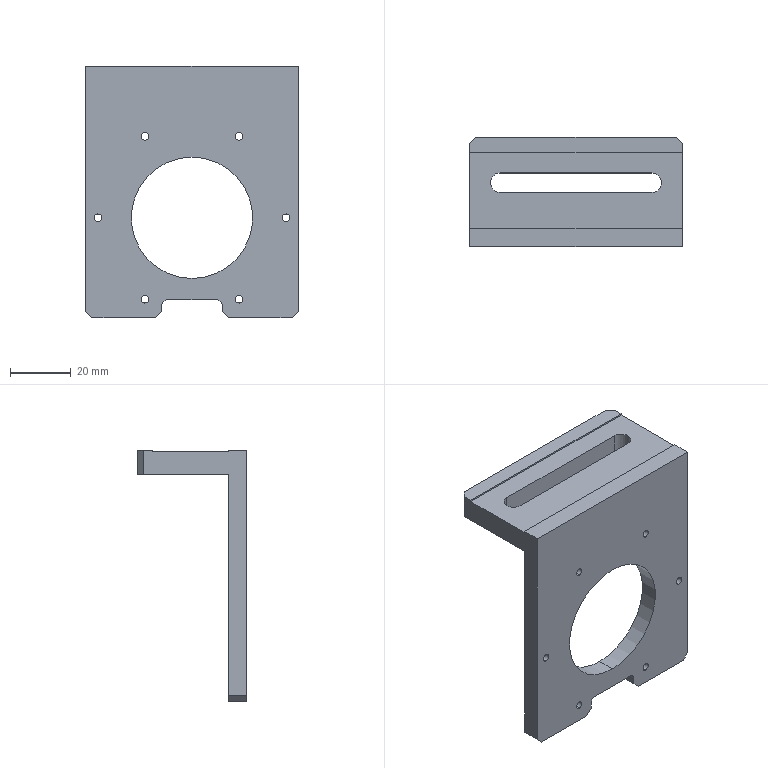Part | SolidWorks | features ICE 6, Chamfer 1, Extrusion 1, Fillet 1 | 1 solid | 43 faces | box 70 x 36 x 83 mm | volume 39637 mm3 | plane 24 | cylinder 19 | commonest cylinder face diameters 2.5 x12 6.4 x3 4 x2 40 x2
STEP:
#1=CARTESIAN_POINT('',(-25.,24.2,41.));
#2=VERTEX_POINT('',#1);
#3=CARTESIAN_POINT('',(-28.2,21.,41.));
#4=VERTEX_POINT('',#3);
#5=CARTESIAN_POINT('',(-25.,21.,41.));
#6=DIRECTION('',(0.,0.,1.));
#7=DIRECTION('',(-1.,0.,0.));
#8=AXIS2_PLACEMENT_3D('',#5,#6,#7);
#9=CIRCLE('',#8,3.2);
#10=EDGE_CURVE('',#2,#4,#9,.T.);
#11=ORIENTED_EDGE('',*,*,#10,.T.);
#12=CARTESIAN_POINT('',(-28.2,21.,33.5));
#13=VERTEX_POINT('',#12);
#14=CARTESIAN_POINT('',(-28.2,21.,53.5));
#15=DIRECTION('',(0.,0.,-1.));
#16=VECTOR('',#15,1000.);
#17=LINE('',#14,#16);
#18=EDGE_CURVE('',#4,#13,#17,.T.);
#19=ORIENTED_EDGE('',*,*,#18,.T.);
#20=CARTESIAN_POINT('',(-25.,24.2,33.5));
#21=VERTEX_POINT('',#20);
#22=CARTESIAN_POINT('',(-25.,21.,33.5));
#23=DIRECTION('',(0.,0.,-1.));
#24=DIRECTION('',(-1.,0.,0.));
#25=AXIS2_PLACEMENT_3D('',#22,#23,#24);
#26=CIRCLE('',#25,3.2);
#27=EDGE_CURVE('',#13,#21,#26,.T.);
#28=ORIENTED_EDGE('',*,*,#27,.T.);
#29=CARTESIAN_POINT('',(-25.,24.2,53.5));
#30=DIRECTION('',(0.,0.,-1.));
#31=VECTOR('',#30,1000.);
#32=LINE('',#29,#31);
#33=EDGE_CURVE('',#2,#21,#32,.T.);
#34=ORIENTED_EDGE('',*,*,#33,.F.);
#35=EDGE_LOOP('',(#11,#19,#28,#34));
#36=FACE_OUTER_BOUND('',#35,.T.);
#37=CARTESIAN_POINT('',(-25.,21.,53.5));
#38=DIRECTION('',(0.,0.,-1.));
#39=DIRECTION('',(-1.,0.,0.));
#40=AXIS2_PLACEMENT_3D('',#37,#38,#39);
#41=CYLINDRICAL_SURFACE('',#40,3.2);
#42=ADVANCED_FACE('',(#36),#41,.F.);
#43=CARTESIAN_POINT('',(31.,0.,-7.25));
#44=VERTEX_POINT('',#43);
#45=CARTESIAN_POINT('',(31.,0.,-9.75));
#46=VERTEX_POINT('',#45);
#47=CARTESIAN_POINT('',(31.,0.,-8.5));
#48=DIRECTION('',(0.,-1.,0.));
#49=DIRECTION('',(0.,0.,-1.));
#50=AXIS2_PLACEMENT_3D('',#47,#48,#49);
#51=CIRCLE('',#50,1.25);
#52=EDGE_CURVE('',#44,#46,#51,.T.);
#53=ORIENTED_EDGE('',*,*,#52,.T.);
#54=CARTESIAN_POINT('',(31.,6.,-9.75));
#55=VERTEX_POINT('',#54);
#56=CARTESIAN_POINT('',(31.,-14.,-9.75));
#57=DIRECTION('',(0.,1.,0.));
#58=VECTOR('',#57,1000.);
#59=LINE('',#56,#58);
#60=EDGE_CURVE('',#46,#55,#59,.T.);
#61=ORIENTED_EDGE('',*,*,#60,.T.);
#62=CARTESIAN_POINT('',(31.,6.,-7.25));
#63=VERTEX_POINT('',#62);
#64=CARTESIAN_POINT('',(31.,6.,-8.5));
#65=DIRECTION('',(0.,1.,0.));
#66=DIRECTION('',(0.,0.,1.));
#67=AXIS2_PLACEMENT_3D('',#64,#65,#66);
#68=CIRCLE('',#67,1.25);
#69=EDGE_CURVE('',#55,#63,#68,.T.);
#70=ORIENTED_EDGE('',*,*,#69,.T.);
#71=CARTESIAN_POINT('',(31.,-14.,-7.25));
#72=DIRECTION('',(0.,1.,0.));
#73=VECTOR('',#72,1000.);
#74=LINE('',#71,#73);
#75=EDGE_CURVE('',#44,#63,#74,.T.);
#76=ORIENTED_EDGE('',*,*,#75,.F.);
#77=EDGE_LOOP('',(#53,#61,#70,#76));
#78=FACE_OUTER_BOUND('',#77,.T.);
#79=CARTESIAN_POINT('',(31.,-14.,-8.5));
#80=DIRECTION('',(0.,1.,0.));
#81=DIRECTION('',(0.,0.,1.));
#82=AXIS2_PLACEMENT_3D('',#79,#80,#81);
#83=CYLINDRICAL_SURFACE('',#82,1.25);
#84=ADVANCED_FACE('',(#78),#83,.F.);
#85=CARTESIAN_POINT('',(15.5,0.,-34.097));
#86=VERTEX_POINT('',#85);
#87=CARTESIAN_POINT('',(15.5,0.,-36.597));
#88=VERTEX_POINT('',#87);
#89=CARTESIAN_POINT('',(15.5,0.,-35.347));
#90=DIRECTION('',(0.,-1.,0.));
#91=DIRECTION('',(0.,0.,-1.));
#92=AXIS2_PLACEMENT_3D('',#89,#90,#91);
#93=CIRCLE('',#92,1.25);
#94=EDGE_CURVE('',#86,#88,#93,.T.);
#95=ORIENTED_EDGE('',*,*,#94,.T.);
#96=CARTESIAN_POINT('',(15.5,6.,-36.597));
#97=VERTEX_POINT('',#96);
#98=CARTESIAN_POINT('',(15.5,-14.,-36.597));
#99=DIRECTION('',(0.,1.,0.));
#100=VECTOR('',#99,1000.);
#101=LINE('',#98,#100);
#102=EDGE_CURVE('',#88,#97,#101,.T.);
#103=ORIENTED_EDGE('',*,*,#102,.T.);
#104=CARTESIAN_POINT('',(15.5,6.,-34.097));
#105=VERTEX_POINT('',#104);
#106=CARTESIAN_POINT('',(15.5,6.,-35.347));
#107=DIRECTION('',(0.,1.,0.));
#108=DIRECTION('',(0.,0.,1.));
#109=AXIS2_PLACEMENT_3D('',#106,#107,#108);
#110=CIRCLE('',#109,1.25);
#111=EDGE_CURVE('',#97,#105,#110,.T.);
#112=ORIENTED_EDGE('',*,*,#111,.T.);
#113=CARTESIAN_POINT('',(15.5,-14.,-34.097));
#114=DIRECTION('',(0.,1.,0.));
#115=VECTOR('',#114,1000.);
#116=LINE('',#113,#115);
#117=EDGE_CURVE('',#86,#105,#116,.T.);
#118=ORIENTED_EDGE('',*,*,#117,.F.);
#119=EDGE_LOOP('',(#95,#103,#112,#118));
#120=FACE_OUTER_BOUND('',#119,.T.);
#121=CARTESIAN_POINT('',(15.5,-14.,-35.347));
#122=DIRECTION('',(0.,1.,0.));
#123=DIRECTION('',(0.,0.,1.));
#124=AXIS2_PLACEMENT_3D('',#121,#122,#123);
#125=CYLINDRICAL_SURFACE('',#124,1.25);
#126=ADVANCED_FACE('',(#120),#125,.F.);
#127=CARTESIAN_POINT('',(-15.5,0.,-34.097));
#128=VERTEX_POINT('',#127);
#129=CARTESIAN_POINT('',(-15.5,0.,-36.597));
#130=VERTEX_POINT('',#129);
#131=CARTESIAN_POINT('',(-15.5,0.,-35.347));
#132=DIRECTION('',(0.,-1.,0.));
#133=DIRECTION('',(0.,0.,-1.));
#134=AXIS2_PLACEMENT_3D('',#131,#132,#133);
#135=CIRCLE('',#134,1.25);
#136=EDGE_CURVE('',#128,#130,#135,.T.);
#137=ORIENTED_EDGE('',*,*,#136,.T.);
#138=CARTESIAN_POINT('',(-15.5,6.,-36.597));
#139=VERTEX_POINT('',#138);
#140=CARTESIAN_POINT('',(-15.5,-14.,-36.597));
#141=DIRECTION('',(0.,1.,0.));
#142=VECTOR('',#141,1000.);
#143=LINE('',#140,#142);
#144=EDGE_CURVE('',#130,#139,#143,.T.);
#145=ORIENTED_EDGE('',*,*,#144,.T.);
#146=CARTESIAN_POINT('',(-15.5,6.,-34.097));
#147=VERTEX_POINT('',#146);
#148=CARTESIAN_POINT('',(-15.5,6.,-35.347));
#149=DIRECTION('',(0.,1.,0.));
#150=DIRECTION('',(0.,0.,1.));
#151=AXIS2_PLACEMENT_3D('',#148,#149,#150);
#152=CIRCLE('',#151,1.25);
#153=EDGE_CURVE('',#139,#147,#152,.T.);
#154=ORIENTED_EDGE('',*,*,#153,.T.);
#155=CARTESIAN_POINT('',(-15.5,-14.,-34.097));
#156=DIRECTION('',(0.,1.,0.));
#157=VECTOR('',#156,1000.);
#158=LINE('',#155,#157);
#159=EDGE_CURVE('',#128,#147,#158,.T.);
#160=ORIENTED_EDGE('',*,*,#159,.F.);
#161=EDGE_LOOP('',(#137,#145,#154,#160));
#162=FACE_OUTER_BOUND('',#161,.T.);
#163=CARTESIAN_POINT('',(-15.5,-14.,-35.347));
#164=DIRECTION('',(0.,1.,0.));
#165=DIRECTION('',(0.,0.,1.));
#166=AXIS2_PLACEMENT_3D('',#163,#164,#165);
#167=CYLINDRICAL_SURFACE('',#166,1.25);
#168=ADVANCED_FACE('',(#162),#167,.F.);
#169=CARTESIAN_POINT('',(-31.,0.,-7.25));
#170=VERTEX_POINT('',#169);
#171=CARTESIAN_POINT('',(-31.,0.,-9.75));
#172=VERTEX_POINT('',#171);
#173=CARTESIAN_POINT('',(-31.,0.,-8.5));
#174=DIRECTION('',(0.,-1.,0.));
#175=DIRECTION('',(0.,0.,-1.));
#176=AXIS2_PLACEMENT_3D('',#173,#174,#175);
#177=CIRCLE('',#176,1.25);
#178=EDGE_CURVE('',#170,#172,#177,.T.);
#179=ORIENTED_EDGE('',*,*,#178,.T.);
#180=CARTESIAN_POINT('',(-31.,6.,-9.75));
#181=VERTEX_POINT('',#180);
#182=CARTESIAN_POINT('',(-31.,-14.,-9.75));
#183=DIRECTION('',(0.,1.,0.));
#184=VECTOR('',#183,1000.);
#185=LINE('',#182,#184);
#186=EDGE_CURVE('',#172,#181,#185,.T.);
#187=ORIENTED_EDGE('',*,*,#186,.T.);
#188=CARTESIAN_POINT('',(-31.,6.,-7.25));
#189=VERTEX_POINT('',#188);
#190=CARTESIAN_POINT('',(-31.,6.,-8.5));
#191=DIRECTION('',(0.,1.,0.));
#192=DIRECTION('',(0.,0.,1.));
#193=AXIS2_PLACEMENT_3D('',#190,#191,#192);
#194=CIRCLE('',#193,1.25);
#195=EDGE_CURVE('',#181,#189,#194,.T.);
#196=ORIENTED_EDGE('',*,*,#195,.T.);
#197=CARTESIAN_POINT('',(-31.,-14.,-7.25));
#198=DIRECTION('',(0.,1.,0.));
#199=VECTOR('',#198,1000.);
#200=LINE('',#197,#199);
#201=EDGE_CURVE('',#170,#189,#200,.T.);
#202=ORIENTED_EDGE('',*,*,#201,.F.);
#203=EDGE_LOOP('',(#179,#187,#196,#202));
#204=FACE_OUTER_BOUND('',#203,.T.);
#205=CARTESIAN_POINT('',(-31.,-14.,-8.5));
#206=DIRECTION('',(0.,1.,0.));
#207=DIRECTION('',(0.,0.,1.));
#208=AXIS2_PLACEMENT_3D('',#205,#206,#207);
#209=CYLINDRICAL_SURFACE('',#208,1.25);
#210=ADVANCED_FACE('',(#204),#209,.F.);
#211=CARTESIAN_POINT('',(-15.5,0.,19.597));
#212=VERTEX_POINT('',#211);
#213=CARTESIAN_POINT('',(-15.5,0.,17.097));
#214=VERTEX_POINT('',#213);
#215=CARTESIAN_POINT('',(-15.5,0.,18.347));
#216=DIRECTION('',(0.,-1.,0.));
#217=DIRECTION('',(0.,0.,-1.));
#218=AXIS2_PLACEMENT_3D('',#215,#216,#217);
#219=CIRCLE('',#218,1.25);
#220=EDGE_CURVE('',#212,#214,#219,.T.);
#221=ORIENTED_EDGE('',*,*,#220,.T.);
#222=CARTESIAN_POINT('',(-15.5,6.,17.097));
#223=VERTEX_POINT('',#222);
#224=CARTESIAN_POINT('',(-15.5,-14.,17.097));
#225=DIRECTION('',(0.,1.,0.));
#226=VECTOR('',#225,1000.);
#227=LINE('',#224,#226);
#228=EDGE_CURVE('',#214,#223,#227,.T.);
#229=ORIENTED_EDGE('',*,*,#228,.T.);
#230=CARTESIAN_POINT('',(-15.5,6.,19.597));
#231=VERTEX_POINT('',#230);
#232=CARTESIAN_POINT('',(-15.5,6.,18.347));
#233=DIRECTION('',(0.,1.,0.));
#234=DIRECTION('',(0.,0.,1.));
#235=AXIS2_PLACEMENT_3D('',#232,#233,#234);
#236=CIRCLE('',#235,1.25);
#237=EDGE_CURVE('',#223,#231,#236,.T.);
#238=ORIENTED_EDGE('',*,*,#237,.T.);
#239=CARTESIAN_POINT('',(-15.5,-14.,19.597));
#240=DIRECTION('',(0.,1.,0.));
#241=VECTOR('',#240,1000.);
#242=LINE('',#239,#241);
#243=EDGE_CURVE('',#212,#231,#242,.T.);
#244=ORIENTED_EDGE('',*,*,#243,.F.);
#245=EDGE_LOOP('',(#221,#229,#238,#244));
#246=FACE_OUTER_BOUND('',#245,.T.);
#247=CARTESIAN_POINT('',(-15.5,-14.,18.347));
#248=DIRECTION('',(0.,1.,0.));
#249=DIRECTION('',(0.,0.,1.));
#250=AXIS2_PLACEMENT_3D('',#247,#248,#249);
#251=CYLINDRICAL_SURFACE('',#250,1.25);
#252=ADVANCED_FACE('',(#246),#251,.F.);
#253=CARTESIAN_POINT('',(15.5,0.,19.597));
#254=VERTEX_POINT('',#253);
#255=CARTESIAN_POINT('',(15.5,0.,17.097));
#256=VERTEX_POINT('',#255);
#257=CARTESIAN_POINT('',(15.5,0.,18.347));
#258=DIRECTION('',(0.,-1.,0.));
#259=DIRECTION('',(0.,0.,-1.));
#260=AXIS2_PLACEMENT_3D('',#257,#258,#259);
#261=CIRCLE('',#260,1.25);
#262=EDGE_CURVE('',#254,#256,#261,.T.);
#263=ORIENTED_EDGE('',*,*,#262,.T.);
#264=CARTESIAN_POINT('',(15.5,6.,17.097));
#265=VERTEX_POINT('',#264);
#266=CARTESIAN_POINT('',(15.5,-14.,17.097));
#267=DIRECTION('',(0.,1.,0.));
#268=VECTOR('',#267,1000.);
#269=LINE('',#266,#268);
#270=EDGE_CURVE('',#256,#265,#269,.T.);
#271=ORIENTED_EDGE('',*,*,#270,.T.);
#272=CARTESIAN_POINT('',(15.5,6.,19.597));
#273=VERTEX_POINT('',#272);
#274=CARTESIAN_POINT('',(15.5,6.,18.347));
#275=DIRECTION('',(0.,1.,0.));
#276=DIRECTION('',(0.,0.,1.));
#277=AXIS2_PLACEMENT_3D('',#274,#275,#276);
#278=CIRCLE('',#277,1.25);
#279=EDGE_CURVE('',#265,#273,#278,.T.);
#280=ORIENTED_EDGE('',*,*,#279,.T.);
#281=CARTESIAN_POINT('',(15.5,-14.,19.597));
#282=DIRECTION('',(0.,1.,0.));
#283=VECTOR('',#282,1000.);
#284=LINE('',#281,#283);
#285=EDGE_CURVE('',#254,#273,#284,.T.);
#286=ORIENTED_EDGE('',*,*,#285,.F.);
#287=EDGE_LOOP('',(#263,#271,#280,#286));
#288=FACE_OUTER_BOUND('',#287,.T.);
#289=CARTESIAN_POINT('',(15.5,-14.,18.347));
#290=DIRECTION('',(0.,1.,0.));
#291=DIRECTION('',(0.,0.,1.));
#292=AXIS2_PLACEMENT_3D('',#289,#290,#291);
#293=CYLINDRICAL_SURFACE('',#292,1.25);
#294=ADVANCED_FACE('',(#288),#293,.F.);
#295=CARTESIAN_POINT('',(0.,6.,11.5));
#296=VERTEX_POINT('',#295);
#297=CARTESIAN_POINT('',(0.,6.,-28.5));
#298=VERTEX_POINT('',#297);
#299=CARTESIAN_POINT('',(0.,6.,-8.5));
#300=DIRECTION('',(0.,-1.,0.));
#301=DIRECTION('',(0.,0.,-1.));
#302=AXIS2_PLACEMENT_3D('',#299,#300,#301);
#303=CIRCLE('',#302,20.);
#304=EDGE_CURVE('',#296,#298,#303,.T.);
#305=ORIENTED_EDGE('',*,*,#304,.F.);
#306=CARTESIAN_POINT('',(0.,0.,11.5));
#307=VERTEX_POINT('',#306);
#308=CARTESIAN_POINT('',(0.,20.,11.5));
#309=DIRECTION('',(0.,-1.,0.));
#310=VECTOR('',#309,1000.);
#311=LINE('',#308,#310);
#312=EDGE_CURVE('',#296,#307,#311,.T.);
#313=ORIENTED_EDGE('',*,*,#312,.T.);
#314=CARTESIAN_POINT('',(0.,0.,-28.5));
#315=VERTEX_POINT('',#314);
#316=CARTESIAN_POINT('',(0.,0.,-8.5));
#317=DIRECTION('',(0.,-1.,0.));
#318=DIRECTION('',(0.,0.,-1.));
#319=AXIS2_PLACEMENT_3D('',#316,#317,#318);
#320=CIRCLE('',#319,20.);
#321=EDGE_CURVE('',#307,#315,#320,.T.);
#322=ORIENTED_EDGE('',*,*,#321,.T.);
#323=CARTESIAN_POINT('',(0.,20.,-28.5));
#324=DIRECTION('',(0.,-1.,0.));
#325=VECTOR('',#324,1000.);
#326=LINE('',#323,#325);
#327=EDGE_CURVE('',#298,#315,#326,.T.);
#328=ORIENTED_EDGE('',*,*,#327,.F.);
#329=EDGE_LOOP('',(#305,#313,#322,#328));
#330=FACE_OUTER_BOUND('',#329,.T.);
#331=CARTESIAN_POINT('',(0.,20.,-8.5));
#332=DIRECTION('',(0.,-1.,0.));
#333=DIRECTION('',(0.,0.,-1.));
#334=AXIS2_PLACEMENT_3D('',#331,#332,#333);
#335=CYLINDRICAL_SURFACE('',#334,20.);
#336=ADVANCED_FACE('',(#330),#335,.F.);
#337=CARTESIAN_POINT('',(35.,6.,41.5));
#338=VERTEX_POINT('',#337);
#339=CARTESIAN_POINT('',(35.,0.,41.5));
#340=VERTEX_POINT('',#339);
#341=CARTESIAN_POINT('',(35.,6.,41.5));
#342=DIRECTION('',(0.,-1.,0.));
#343=VECTOR('',#342,1000.);
#344=LINE('',#341,#343);
#345=EDGE_CURVE('',#338,#340,#344,.T.);
#346=ORIENTED_EDGE('',*,*,#345,.F.);
#347=CARTESIAN_POINT('',(-35.,6.,41.5));
#348=VERTEX_POINT('',#347);
#349=CARTESIAN_POINT('',(55.,6.,41.5));
#350=DIRECTION('',(-1.,0.,0.));
#351=VECTOR('',#350,1000.);
#352=LINE('',#349,#351);
#353=EDGE_CURVE('',#338,#348,#352,.T.);
#354=ORIENTED_EDGE('',*,*,#353,.T.);
#355=CARTESIAN_POINT('',(-35.,0.,41.5));
#356=VERTEX_POINT('',#355);
#357=CARTESIAN_POINT('',(-35.,6.,41.5));
#358=DIRECTION('',(0.,-1.,0.));
#359=VECTOR('',#358,1000.);
#360=LINE('',#357,#359);
#361=EDGE_CURVE('',#348,#356,#360,.T.);
#362=ORIENTED_EDGE('',*,*,#361,.T.);
#363=CARTESIAN_POINT('',(-35.,0.,41.5));
#364=DIRECTION('',(1.,0.,0.));
#365=VECTOR('',#364,1000.);
#366=LINE('',#363,#365);
#367=EDGE_CURVE('',#356,#340,#366,.T.);
#368=ORIENTED_EDGE('',*,*,#367,.T.);
#369=EDGE_LOOP('',(#346,#354,#362,#368));
#370=FACE_OUTER_BOUND('',#369,.T.);
#371=CARTESIAN_POINT('',(-35.,6.,41.5));
#372=DIRECTION('',(0.,0.,-1.));
#373=DIRECTION('',(-1.,0.,0.));
#374=AXIS2_PLACEMENT_3D('',#371,#372,#373);
#375=PLANE('',#374);
#376=ADVANCED_FACE('',(#370),#375,.F.);
#377=CARTESIAN_POINT('',(-12.,6.,-41.5));
#378=VERTEX_POINT('',#377);
#379=CARTESIAN_POINT('',(-33.,6.,-41.5));
#380=VERTEX_POINT('',#379);
#381=CARTESIAN_POINT('',(-35.,6.,-41.5));
#382=DIRECTION('',(-1.,0.,0.));
#383=VECTOR('',#382,1000.);
#384=LINE('',#381,#383);
#385=EDGE_CURVE('',#378,#380,#384,.T.);
#386=ORIENTED_EDGE('',*,*,#385,.F.);
#387=CARTESIAN_POINT('',(-12.,0.,-41.5));
#388=VERTEX_POINT('',#387);
#389=CARTESIAN_POINT('',(-12.,6.,-41.5));
#390=DIRECTION('',(0.,-1.,0.));
#391=VECTOR('',#390,1000.);
#392=LINE('',#389,#391);
#393=EDGE_CURVE('',#378,#388,#392,.T.);
#394=ORIENTED_EDGE('',*,*,#393,.T.);
#395=CARTESIAN_POINT('',(-33.,0.,-41.5));
#396=VERTEX_POINT('',#395);
#397=CARTESIAN_POINT('',(-35.,0.,-41.5));
#398=DIRECTION('',(-1.,0.,0.));
#399=VECTOR('',#398,1000.);
#400=LINE('',#397,#399);
#401=EDGE_CURVE('',#388,#396,#400,.T.);
#402=ORIENTED_EDGE('',*,*,#401,.T.);
#403=CARTESIAN_POINT('',(-33.,6.,-41.5));
#404=DIRECTION('',(0.,1.,0.));
#405=VECTOR('',#404,1000.);
#406=LINE('',#403,#405);
#407=EDGE_CURVE('',#396,#380,#406,.T.);
#408=ORIENTED_EDGE('',*,*,#407,.T.);
#409=EDGE_LOOP('',(#386,#394,#402,#408));
#410=FACE_OUTER_BOUND('',#409,.T.);
#411=CARTESIAN_POINT('',(-35.,6.,-41.5));
#412=DIRECTION('',(0.,0.,1.));
#413=DIRECTION('',(1.,0.,0.));
#414=AXIS2_PLACEMENT_3D('',#411,#412,#413);
#415=PLANE('',#414);
#416=ADVANCED_FACE('',(#410),#415,.F.);
#417=CARTESIAN_POINT('',(31.,6.,-8.5));
#418=DIRECTION('',(0.,1.,0.));
#419=DIRECTION('',(0.,0.,1.));
#420=AXIS2_PLACEMENT_3D('',#417,#418,#419);
#421=CIRCLE('',#420,1.25);
#422=EDGE_CURVE('',#63,#55,#421,.T.);
#423=ORIENTED_EDGE('',*,*,#422,.F.);
#424=ORIENTED_EDGE('',*,*,#69,.F.);
#425=EDGE_LOOP('',(#423,#424));
#426=FACE_BOUND('',#425,.T.);
#427=CARTESIAN_POINT('',(15.5,6.,-35.347));
#428=DIRECTION('',(0.,1.,0.));
#429=DIRECTION('',(0.,0.,1.));
#430=AXIS2_PLACEMENT_3D('',#427,#428,#429);
#431=CIRCLE('',#430,1.25);
#432=EDGE_CURVE('',#105,#97,#431,.T.);
#433=ORIENTED_EDGE('',*,*,#432,.F.);
#434=ORIENTED_EDGE('',*,*,#111,.F.);
#435=EDGE_LOOP('',(#433,#434));
#436=FACE_BOUND('',#435,.T.);
#437=CARTESIAN_POINT('',(-15.5,6.,-35.347));
#438=DIRECTION('',(0.,1.,0.));
#439=DIRECTION('',(0.,0.,1.));
#440=AXIS2_PLACEMENT_3D('',#437,#438,#439);
#441=CIRCLE('',#440,1.25);
#442=EDGE_CURVE('',#147,#139,#441,.T.);
#443=ORIENTED_EDGE('',*,*,#442,.F.);
#444=ORIENTED_EDGE('',*,*,#153,.F.);
#445=EDGE_LOOP('',(#443,#444));
#446=FACE_BOUND('',#445,.T.);
#447=CARTESIAN_POINT('',(-31.,6.,-8.5));
#448=DIRECTION('',(0.,1.,0.));
#449=DIRECTION('',(0.,0.,1.));
#450=AXIS2_PLACEMENT_3D('',#447,#448,#449);
#451=CIRCLE('',#450,1.25);
#452=EDGE_CURVE('',#189,#181,#451,.T.);
#453=ORIENTED_EDGE('',*,*,#452,.F.);
#454=ORIENTED_EDGE('',*,*,#195,.F.);
#455=EDGE_LOOP('',(#453,#454));
#456=FACE_BOUND('',#455,.T.);
#457=CARTESIAN_POINT('',(-15.5,6.,18.347));
#458=DIRECTION('',(0.,1.,0.));
#459=DIRECTION('',(0.,0.,1.));
#460=AXIS2_PLACEMENT_3D('',#457,#458,#459);
#461=CIRCLE('',#460,1.25);
#462=EDGE_CURVE('',#231,#223,#461,.T.);
#463=ORIENTED_EDGE('',*,*,#462,.F.);
#464=ORIENTED_EDGE('',*,*,#237,.F.);
#465=EDGE_LOOP('',(#463,#464));
#466=FACE_BOUND('',#465,.T.);
#467=CARTESIAN_POINT('',(15.5,6.,18.347));
#468=DIRECTION('',(0.,1.,0.));
#469=DIRECTION('',(0.,0.,1.));
#470=AXIS2_PLACEMENT_3D('',#467,#468,#469);
#471=CIRCLE('',#470,1.25);
#472=EDGE_CURVE('',#273,#265,#471,.T.);
#473=ORIENTED_EDGE('',*,*,#472,.F.);
#474=ORIENTED_EDGE('',*,*,#279,.F.);
#475=EDGE_LOOP('',(#473,#474));
#476=FACE_BOUND('',#475,.T.);
#477=CARTESIAN_POINT('',(0.,6.,-8.5));
#478=DIRECTION('',(0.,-1.,0.));
#479=DIRECTION('',(0.,0.,-1.));
#480=AXIS2_PLACEMENT_3D('',#477,#478,#479);
#481=CIRCLE('',#480,20.);
#482=EDGE_CURVE('',#298,#296,#481,.T.);
#483=ORIENTED_EDGE('',*,*,#482,.T.);
#484=ORIENTED_EDGE('',*,*,#304,.T.);
#485=EDGE_LOOP('',(#483,#484));
#486=FACE_BOUND('',#485,.T.);
#487=CARTESIAN_POINT('',(33.,6.,-41.5));
#488=VERTEX_POINT('',#487);
#489=CARTESIAN_POINT('',(12.,6.,-41.5));
#490=VERTEX_POINT('',#489);
#491=CARTESIAN_POINT('',(-35.,6.,-41.5));
#492=DIRECTION('',(-1.,0.,0.));
#493=VECTOR('',#492,1000.);
#494=LINE('',#491,#493);
#495=EDGE_CURVE('',#488,#490,#494,.T.);
#496=ORIENTED_EDGE('',*,*,#495,.T.);
#497=CARTESIAN_POINT('',(10.,6.,-39.5));
#498=VERTEX_POINT('',#497);
#499=CARTESIAN_POINT('',(12.,6.,-41.5));
#500=DIRECTION('',(-0.7071,0.,0.7071));
#501=VECTOR('',#500,1000.);
#502=LINE('',#499,#501);
#503=EDGE_CURVE('',#490,#498,#502,.T.);
#504=ORIENTED_EDGE('',*,*,#503,.T.);
#505=CARTESIAN_POINT('',(10.,6.,-37.5));
#506=VERTEX_POINT('',#505);
#507=CARTESIAN_POINT('',(10.,6.,-47.519));
#508=DIRECTION('',(0.,0.,-1.));
#509=VECTOR('',#508,1000.);
#510=LINE('',#507,#509);
#511=EDGE_CURVE('',#506,#498,#510,.T.);
#512=ORIENTED_EDGE('',*,*,#511,.F.);
#513=CARTESIAN_POINT('',(8.,6.,-35.5));
#514=VERTEX_POINT('',#513);
#515=CARTESIAN_POINT('',(8.,6.,-37.5));
#516=DIRECTION('',(0.,-1.,0.));
#517=DIRECTION('',(0.,0.,-1.));
#518=AXIS2_PLACEMENT_3D('',#515,#516,#517);
#519=CIRCLE('',#518,2.);
#520=EDGE_CURVE('',#506,#514,#519,.T.);
#521=ORIENTED_EDGE('',*,*,#520,.T.);
#522=CARTESIAN_POINT('',(-8.,6.,-35.5));
#523=VERTEX_POINT('',#522);
#524=CARTESIAN_POINT('',(-10.,6.,-35.5));
#525=DIRECTION('',(1.,0.,0.));
#526=VECTOR('',#525,1000.);
#527=LINE('',#524,#526);
#528=EDGE_CURVE('',#523,#514,#527,.T.);
#529=ORIENTED_EDGE('',*,*,#528,.F.);
#530=CARTESIAN_POINT('',(-10.,6.,-37.5));
#531=VERTEX_POINT('',#530);
#532=CARTESIAN_POINT('',(-8.,6.,-37.5));
#533=DIRECTION('',(0.,-1.,0.));
#534=DIRECTION('',(0.,0.,-1.));
#535=AXIS2_PLACEMENT_3D('',#532,#533,#534);
#536=CIRCLE('',#535,2.);
#537=EDGE_CURVE('',#523,#531,#536,.T.);
#538=ORIENTED_EDGE('',*,*,#537,.T.);
#539=CARTESIAN_POINT('',(-10.,6.,-39.5));
#540=VERTEX_POINT('',#539);
#541=CARTESIAN_POINT('',(-10.,6.,-47.519));
#542=DIRECTION('',(0.,0.,1.));
#543=VECTOR('',#542,1000.);
#544=LINE('',#541,#543);
#545=EDGE_CURVE('',#540,#531,#544,.T.);
#546=ORIENTED_EDGE('',*,*,#545,.F.);
#547=CARTESIAN_POINT('',(-12.,6.,-41.5));
#548=DIRECTION('',(-0.7071,0.,-0.7071));
#549=VECTOR('',#548,1000.);
#550=LINE('',#547,#549);
#551=EDGE_CURVE('',#540,#378,#550,.T.);
#552=ORIENTED_EDGE('',*,*,#551,.T.);
#553=ORIENTED_EDGE('',*,*,#385,.T.);
#554=CARTESIAN_POINT('',(-35.,6.,-39.5));
#555=VERTEX_POINT('',#554);
#556=CARTESIAN_POINT('',(-35.,6.,-39.5));
#557=DIRECTION('',(-0.7071,0.,0.7071));
#558=VECTOR('',#557,1000.);
#559=LINE('',#556,#558);
#560=EDGE_CURVE('',#380,#555,#559,.T.);
#561=ORIENTED_EDGE('',*,*,#560,.T.);
#562=CARTESIAN_POINT('',(-35.,6.,33.5));
#563=VERTEX_POINT('',#562);
#564=CARTESIAN_POINT('',(-35.,6.,41.5));
#565=DIRECTION('',(0.,0.,1.));
#566=VECTOR('',#565,1000.);
#567=LINE('',#564,#566);
#568=EDGE_CURVE('',#555,#563,#567,.T.);
#569=ORIENTED_EDGE('',*,*,#568,.T.);
#570=CARTESIAN_POINT('',(35.,6.,33.5));
#571=VERTEX_POINT('',#570);
#572=CARTESIAN_POINT('',(-35.,6.,33.5));
#573=DIRECTION('',(-1.,0.,0.));
#574=VECTOR('',#573,1000.);
#575=LINE('',#572,#574);
#576=EDGE_CURVE('',#571,#563,#575,.T.);
#577=ORIENTED_EDGE('',*,*,#576,.F.);
#578=CARTESIAN_POINT('',(35.,6.,-39.5));
#579=VERTEX_POINT('',#578);
#580=CARTESIAN_POINT('',(35.,6.,41.5));
#581=DIRECTION('',(0.,0.,-1.));
#582=VECTOR('',#581,1000.);
#583=LINE('',#580,#582);
#584=EDGE_CURVE('',#571,#579,#583,.T.);
#585=ORIENTED_EDGE('',*,*,#584,.T.);
#586=CARTESIAN_POINT('',(33.,6.,-41.5));
#587=DIRECTION('',(-0.7071,0.,-0.7071));
#588=VECTOR('',#587,1000.);
#589=LINE('',#586,#588);
#590=EDGE_CURVE('',#579,#488,#589,.T.);
#591=ORIENTED_EDGE('',*,*,#590,.T.);
#592=EDGE_LOOP('',(#496,#504,#512,#521,#529,#538,#546,#552,#553,#561,#569,#577,#585,#591));
#593=FACE_OUTER_BOUND('',#592,.T.);
#594=CARTESIAN_POINT('',(0.,6.,0.));
#595=DIRECTION('',(0.,-1.,0.));
#596=DIRECTION('',(0.,0.,-1.));
#597=AXIS2_PLACEMENT_3D('',#594,#595,#596);
#598=PLANE('',#597);
#599=ADVANCED_FACE('',(#426,#436,#446,#456,#466,#476,#486,#593),#598,.F.);
#600=CARTESIAN_POINT('',(35.,34.,33.5));
#601=VERTEX_POINT('',#600);
#602=CARTESIAN_POINT('',(35.,36.,33.5));
#603=DIRECTION('',(0.,-1.,0.));
#604=VECTOR('',#603,1000.);
#605=LINE('',#602,#604);
#606=EDGE_CURVE('',#601,#571,#605,.T.);
#607=ORIENTED_EDGE('',*,*,#606,.F.);
#608=CARTESIAN_POINT('',(35.,34.,41.5));
#609=VERTEX_POINT('',#608);
#610=CARTESIAN_POINT('',(35.,34.,41.5));
#611=DIRECTION('',(0.,0.,1.));
#612=VECTOR('',#611,1000.);
#613=LINE('',#610,#612);
#614=EDGE_CURVE('',#601,#609,#613,.T.);
#615=ORIENTED_EDGE('',*,*,#614,.T.);
#616=CARTESIAN_POINT('',(35.,31.,41.5));
#617=VERTEX_POINT('',#616);
#618=CARTESIAN_POINT('',(35.,6.,41.5));
#619=DIRECTION('',(0.,-1.,0.));
#620=VECTOR('',#619,1000.);
#621=LINE('',#618,#620);
#622=EDGE_CURVE('',#609,#617,#621,.T.);
#623=ORIENTED_EDGE('',*,*,#622,.T.);
#624=CARTESIAN_POINT('',(35.,31.,41.));
#625=VERTEX_POINT('',#624);
#626=CARTESIAN_POINT('',(35.,31.,41.5));
#627=DIRECTION('',(0.,0.,-1.));
#628=VECTOR('',#627,1000.);
#629=LINE('',#626,#628);
#630=EDGE_CURVE('',#617,#625,#629,.T.);
#631=ORIENTED_EDGE('',*,*,#630,.T.);
#632=CARTESIAN_POINT('',(35.,6.,41.));
#633=VERTEX_POINT('',#632);
#634=CARTESIAN_POINT('',(35.,6.,41.));
#635=DIRECTION('',(0.,-1.,0.));
#636=VECTOR('',#635,1000.);
#637=LINE('',#634,#636);
#638=EDGE_CURVE('',#625,#633,#637,.T.);
#639=ORIENTED_EDGE('',*,*,#638,.T.);
#640=CARTESIAN_POINT('',(35.,6.,41.5));
#641=DIRECTION('',(0.,0.,1.));
#642=VECTOR('',#641,1000.);
#643=LINE('',#640,#642);
#644=EDGE_CURVE('',#633,#338,#643,.T.);
#645=ORIENTED_EDGE('',*,*,#644,.T.);
#646=ORIENTED_EDGE('',*,*,#345,.T.);
#647=CARTESIAN_POINT('',(35.,0.,-39.5));
#648=VERTEX_POINT('',#647);
#649=CARTESIAN_POINT('',(35.,0.,41.5));
#650=DIRECTION('',(0.,0.,-1.));
#651=VECTOR('',#650,1000.);
#652=LINE('',#649,#651);
#653=EDGE_CURVE('',#340,#648,#652,.T.);
#654=ORIENTED_EDGE('',*,*,#653,.T.);
#655=CARTESIAN_POINT('',(35.,6.,-39.5));
#656=DIRECTION('',(0.,1.,0.));
#657=VECTOR('',#656,1000.);
#658=LINE('',#655,#657);
#659=EDGE_CURVE('',#648,#579,#658,.T.);
#660=ORIENTED_EDGE('',*,*,#659,.T.);
#661=ORIENTED_EDGE('',*,*,#584,.F.);
#662=EDGE_LOOP('',(#607,#615,#623,#631,#639,#645,#646,#654,#660,#661));
#663=FACE_OUTER_BOUND('',#662,.T.);
#664=CARTESIAN_POINT('',(35.,6.,41.5));
#665=DIRECTION('',(-1.,0.,0.));
#666=DIRECTION('',(0.,0.,1.));
#667=AXIS2_PLACEMENT_3D('',#664,#665,#666);
#668=PLANE('',#667);
#669=ADVANCED_FACE('',(#663),#668,.F.);
#670=CARTESIAN_POINT('',(33.,0.,-41.5));
#671=VERTEX_POINT('',#670);
#672=CARTESIAN_POINT('',(12.,0.,-41.5));
#673=VERTEX_POINT('',#672);
#674=CARTESIAN_POINT('',(-35.,0.,-41.5));
#675=DIRECTION('',(-1.,0.,0.));
#676=VECTOR('',#675,1000.);
#677=LINE('',#674,#676);
#678=EDGE_CURVE('',#671,#673,#677,.T.);
#679=ORIENTED_EDGE('',*,*,#678,.T.);
#680=CARTESIAN_POINT('',(12.,6.,-41.5));
#681=DIRECTION('',(0.,1.,0.));
#682=VECTOR('',#681,1000.);
#683=LINE('',#680,#682);
#684=EDGE_CURVE('',#673,#490,#683,.T.);
#685=ORIENTED_EDGE('',*,*,#684,.T.);
#686=ORIENTED_EDGE('',*,*,#495,.F.);
#687=CARTESIAN_POINT('',(33.,6.,-41.5));
#688=DIRECTION('',(0.,-1.,0.));
#689=VECTOR('',#688,1000.);
#690=LINE('',#687,#689);
#691=EDGE_CURVE('',#488,#671,#690,.T.);
#692=ORIENTED_EDGE('',*,*,#691,.T.);
#693=EDGE_LOOP('',(#679,#685,#686,#692));
#694=FACE_OUTER_BOUND('',#693,.T.);
#695=CARTESIAN_POINT('',(-35.,6.,-41.5));
#696=DIRECTION('',(0.,0.,1.));
#697=DIRECTION('',(1.,0.,0.));
#698=AXIS2_PLACEMENT_3D('',#695,#696,#697);
#699=PLANE('',#698);
#700=ADVANCED_FACE('',(#694),#699,.F.);
#701=CARTESIAN_POINT('',(-35.,34.,41.5));
#702=VERTEX_POINT('',#701);
#703=CARTESIAN_POINT('',(-35.,31.,41.5));
#704=VERTEX_POINT('',#703);
#705=CARTESIAN_POINT('',(-35.,6.,41.5));
#706=DIRECTION('',(0.,-1.,0.));
#707=VECTOR('',#706,1000.);
#708=LINE('',#705,#707);
#709=EDGE_CURVE('',#702,#704,#708,.T.);
#710=ORIENTED_EDGE('',*,*,#709,.F.);
#711=CARTESIAN_POINT('',(-35.,34.,33.5));
#712=VERTEX_POINT('',#711);
#713=CARTESIAN_POINT('',(-35.,34.,41.5));
#714=DIRECTION('',(0.,0.,-1.));
#715=VECTOR('',#714,1000.);
#716=LINE('',#713,#715);
#717=EDGE_CURVE('',#702,#712,#716,.T.);
#718=ORIENTED_EDGE('',*,*,#717,.T.);
#719=CARTESIAN_POINT('',(-35.,36.,33.5));
#720=DIRECTION('',(0.,-1.,0.));
#721=VECTOR('',#720,1000.);
#722=LINE('',#719,#721);
#723=EDGE_CURVE('',#712,#563,#722,.T.);
#724=ORIENTED_EDGE('',*,*,#723,.T.);
#725=ORIENTED_EDGE('',*,*,#568,.F.);
#726=CARTESIAN_POINT('',(-35.,0.,-39.5));
#727=VERTEX_POINT('',#726);
#728=CARTESIAN_POINT('',(-35.,6.,-39.5));
#729=DIRECTION('',(0.,-1.,0.));
#730=VECTOR('',#729,1000.);
#731=LINE('',#728,#730);
#732=EDGE_CURVE('',#555,#727,#731,.T.);
#733=ORIENTED_EDGE('',*,*,#732,.T.);
#734=CARTESIAN_POINT('',(-35.,0.,41.5));
#735=DIRECTION('',(0.,0.,1.));
#736=VECTOR('',#735,1000.);
#737=LINE('',#734,#736);
#738=EDGE_CURVE('',#727,#356,#737,.T.);
#739=ORIENTED_EDGE('',*,*,#738,.T.);
#740=ORIENTED_EDGE('',*,*,#361,.F.);
#741=CARTESIAN_POINT('',(-35.,6.,41.));
#742=VERTEX_POINT('',#741);
#743=CARTESIAN_POINT('',(-35.,6.,41.5));
#744=DIRECTION('',(0.,0.,1.));
#745=VECTOR('',#744,1000.);
#746=LINE('',#743,#745);
#747=EDGE_CURVE('',#742,#348,#746,.T.);
#748=ORIENTED_EDGE('',*,*,#747,.F.);
#749=CARTESIAN_POINT('',(-35.,31.,41.));
#750=VERTEX_POINT('',#749);
#751=CARTESIAN_POINT('',(-35.,6.,41.));
#752=DIRECTION('',(0.,-1.,0.));
#753=VECTOR('',#752,1000.);
#754=LINE('',#751,#753);
#755=EDGE_CURVE('',#750,#742,#754,.T.);
#756=ORIENTED_EDGE('',*,*,#755,.F.);
#757=CARTESIAN_POINT('',(-35.,31.,41.5));
#758=DIRECTION('',(0.,0.,-1.));
#759=VECTOR('',#758,1000.);
#760=LINE('',#757,#759);
#761=EDGE_CURVE('',#704,#750,#760,.T.);
#762=ORIENTED_EDGE('',*,*,#761,.F.);
#763=EDGE_LOOP('',(#710,#718,#724,#725,#733,#739,#740,#748,#756,#762));
#764=FACE_OUTER_BOUND('',#763,.T.);
#765=CARTESIAN_POINT('',(-35.,6.,41.5));
#766=DIRECTION('',(1.,0.,0.));
#767=DIRECTION('',(0.,0.,-1.));
#768=AXIS2_PLACEMENT_3D('',#765,#766,#767);
#769=PLANE('',#768);
#770=ADVANCED_FACE('',(#764),#769,.F.);
#771=CARTESIAN_POINT('',(-33.,36.,41.5));
#772=VERTEX_POINT('',#771);
#773=CARTESIAN_POINT('',(33.,36.,41.5));
#774=VERTEX_POINT('',#773);
#775=CARTESIAN_POINT('',(-35.,36.,41.5));
#776=DIRECTION('',(1.,0.,0.));
#777=VECTOR('',#776,1000.);
#778=LINE('',#775,#777);
#779=EDGE_CURVE('',#772,#774,#778,.T.);
#780=ORIENTED_EDGE('',*,*,#779,.F.);
#781=CARTESIAN_POINT('',(-33.,36.,41.5));
#782=DIRECTION('',(-0.7071,-0.7071,0.));
#783=VECTOR('',#782,1000.);
#784=LINE('',#781,#783);
#785=EDGE_CURVE('',#772,#702,#784,.T.);
#786=ORIENTED_EDGE('',*,*,#785,.T.);
#787=ORIENTED_EDGE('',*,*,#709,.T.);
#788=CARTESIAN_POINT('',(55.,31.,41.5));
#789=DIRECTION('',(-1.,0.,0.));
#790=VECTOR('',#789,1000.);
#791=LINE('',#788,#790);
#792=EDGE_CURVE('',#617,#704,#791,.T.);
#793=ORIENTED_EDGE('',*,*,#792,.F.);
#794=ORIENTED_EDGE('',*,*,#622,.F.);
#795=CARTESIAN_POINT('',(33.,36.,41.5));
#796=DIRECTION('',(-0.7071,0.7071,0.));
#797=VECTOR('',#796,1000.);
#798=LINE('',#795,#797);
#799=EDGE_CURVE('',#609,#774,#798,.T.);
#800=ORIENTED_EDGE('',*,*,#799,.T.);
#801=EDGE_LOOP('',(#780,#786,#787,#793,#794,#800));
#802=FACE_OUTER_BOUND('',#801,.T.);
#803=CARTESIAN_POINT('',(-35.,6.,41.5));
#804=DIRECTION('',(0.,0.,-1.));
#805=DIRECTION('',(-1.,0.,0.));
#806=AXIS2_PLACEMENT_3D('',#803,#804,#805);
#807=PLANE('',#806);
#808=ADVANCED_FACE('',(#802),#807,.F.);
#809=ORIENTED_EDGE('',*,*,#52,.F.);
#810=CARTESIAN_POINT('',(31.,0.,-8.5));
#811=DIRECTION('',(0.,-1.,0.));
#812=DIRECTION('',(0.,0.,-1.));
#813=AXIS2_PLACEMENT_3D('',#810,#811,#812);
#814=CIRCLE('',#813,1.25);
#815=EDGE_CURVE('',#46,#44,#814,.T.);
#816=ORIENTED_EDGE('',*,*,#815,.F.);
#817=EDGE_LOOP('',(#809,#816));
#818=FACE_BOUND('',#817,.T.);
#819=ORIENTED_EDGE('',*,*,#94,.F.);
#820=CARTESIAN_POINT('',(15.5,0.,-35.347));
#821=DIRECTION('',(0.,-1.,0.));
#822=DIRECTION('',(0.,0.,-1.));
#823=AXIS2_PLACEMENT_3D('',#820,#821,#822);
#824=CIRCLE('',#823,1.25);
#825=EDGE_CURVE('',#88,#86,#824,.T.);
#826=ORIENTED_EDGE('',*,*,#825,.F.);
#827=EDGE_LOOP('',(#819,#826));
#828=FACE_BOUND('',#827,.T.);
#829=ORIENTED_EDGE('',*,*,#136,.F.);
#830=CARTESIAN_POINT('',(-15.5,0.,-35.347));
#831=DIRECTION('',(0.,-1.,0.));
#832=DIRECTION('',(0.,0.,-1.));
#833=AXIS2_PLACEMENT_3D('',#830,#831,#832);
#834=CIRCLE('',#833,1.25);
#835=EDGE_CURVE('',#130,#128,#834,.T.);
#836=ORIENTED_EDGE('',*,*,#835,.F.);
#837=EDGE_LOOP('',(#829,#836));
#838=FACE_BOUND('',#837,.T.);
#839=ORIENTED_EDGE('',*,*,#178,.F.);
#840=CARTESIAN_POINT('',(-31.,0.,-8.5));
#841=DIRECTION('',(0.,-1.,0.));
#842=DIRECTION('',(0.,0.,-1.));
#843=AXIS2_PLACEMENT_3D('',#840,#841,#842);
#844=CIRCLE('',#843,1.25);
#845=EDGE_CURVE('',#172,#170,#844,.T.);
#846=ORIENTED_EDGE('',*,*,#845,.F.);
#847=EDGE_LOOP('',(#839,#846));
#848=FACE_BOUND('',#847,.T.);
#849=ORIENTED_EDGE('',*,*,#220,.F.);
#850=CARTESIAN_POINT('',(-15.5,0.,18.347));
#851=DIRECTION('',(0.,-1.,0.));
#852=DIRECTION('',(0.,0.,-1.));
#853=AXIS2_PLACEMENT_3D('',#850,#851,#852);
#854=CIRCLE('',#853,1.25);
#855=EDGE_CURVE('',#214,#212,#854,.T.);
#856=ORIENTED_EDGE('',*,*,#855,.F.);
#857=EDGE_LOOP('',(#849,#856));
#858=FACE_BOUND('',#857,.T.);
#859=ORIENTED_EDGE('',*,*,#262,.F.);
#860=CARTESIAN_POINT('',(15.5,0.,18.347));
#861=DIRECTION('',(0.,-1.,0.));
#862=DIRECTION('',(0.,0.,-1.));
#863=AXIS2_PLACEMENT_3D('',#860,#861,#862);
#864=CIRCLE('',#863,1.25);
#865=EDGE_CURVE('',#256,#254,#864,.T.);
#866=ORIENTED_EDGE('',*,*,#865,.F.);
#867=EDGE_LOOP('',(#859,#866));
#868=FACE_BOUND('',#867,.T.);
#869=CARTESIAN_POINT('',(10.,0.,-39.5));
#870=VERTEX_POINT('',#869);
#871=CARTESIAN_POINT('',(10.,0.,-37.5));
#872=VERTEX_POINT('',#871);
#873=CARTESIAN_POINT('',(10.,0.,0.));
#874=DIRECTION('',(0.,0.,1.));
#875=VECTOR('',#874,1000.);
#876=LINE('',#873,#875);
#877=EDGE_CURVE('',#870,#872,#876,.T.);
#878=ORIENTED_EDGE('',*,*,#877,.F.);
#879=CARTESIAN_POINT('',(-14.75,0.,-14.75));
#880=DIRECTION('',(0.7071,0.,-0.7071));
#881=VECTOR('',#880,1000.);
#882=LINE('',#879,#881);
#883=EDGE_CURVE('',#870,#673,#882,.T.);
#884=ORIENTED_EDGE('',*,*,#883,.T.);
#885=ORIENTED_EDGE('',*,*,#678,.F.);
#886=CARTESIAN_POINT('',(37.25,0.,-37.25));
#887=DIRECTION('',(0.7071,0.,0.7071));
#888=VECTOR('',#887,1000.);
#889=LINE('',#886,#888);
#890=EDGE_CURVE('',#671,#648,#889,.T.);
#891=ORIENTED_EDGE('',*,*,#890,.T.);
#892=ORIENTED_EDGE('',*,*,#653,.F.);
#893=ORIENTED_EDGE('',*,*,#367,.F.);
#894=ORIENTED_EDGE('',*,*,#738,.F.);
#895=CARTESIAN_POINT('',(-37.25,0.,-37.25));
#896=DIRECTION('',(0.7071,0.,-0.7071));
#897=VECTOR('',#896,1000.);
#898=LINE('',#895,#897);
#899=EDGE_CURVE('',#727,#396,#898,.T.);
#900=ORIENTED_EDGE('',*,*,#899,.T.);
#901=ORIENTED_EDGE('',*,*,#401,.F.);
#902=CARTESIAN_POINT('',(-10.,0.,-39.5));
#903=VERTEX_POINT('',#902);
#904=CARTESIAN_POINT('',(14.75,0.,-14.75));
#905=DIRECTION('',(0.7071,0.,0.7071));
#906=VECTOR('',#905,1000.);
#907=LINE('',#904,#906);
#908=EDGE_CURVE('',#388,#903,#907,.T.);
#909=ORIENTED_EDGE('',*,*,#908,.T.);
#910=CARTESIAN_POINT('',(-10.,0.,-37.5));
#911=VERTEX_POINT('',#910);
#912=CARTESIAN_POINT('',(-10.,0.,0.));
#913=DIRECTION('',(0.,0.,-1.));
#914=VECTOR('',#913,1000.);
#915=LINE('',#912,#914);
#916=EDGE_CURVE('',#911,#903,#915,.T.);
#917=ORIENTED_EDGE('',*,*,#916,.F.);
#918=CARTESIAN_POINT('',(-8.,0.,-35.5));
#919=VERTEX_POINT('',#918);
#920=CARTESIAN_POINT('',(-8.,0.,-37.5));
#921=DIRECTION('',(0.,1.,0.));
#922=DIRECTION('',(0.,0.,-1.));
#923=AXIS2_PLACEMENT_3D('',#920,#921,#922);
#924=CIRCLE('',#923,2.);
#925=EDGE_CURVE('',#911,#919,#924,.T.);
#926=ORIENTED_EDGE('',*,*,#925,.T.);
#927=CARTESIAN_POINT('',(8.,0.,-35.5));
#928=VERTEX_POINT('',#927);
#929=CARTESIAN_POINT('',(0.,0.,-35.5));
#930=DIRECTION('',(-1.,0.,0.));
#931=VECTOR('',#930,1000.);
#932=LINE('',#929,#931);
#933=EDGE_CURVE('',#928,#919,#932,.T.);
#934=ORIENTED_EDGE('',*,*,#933,.F.);
#935=CARTESIAN_POINT('',(8.,0.,-37.5));
#936=DIRECTION('',(0.,1.,0.));
#937=DIRECTION('',(0.,0.,-1.));
#938=AXIS2_PLACEMENT_3D('',#935,#936,#937);
#939=CIRCLE('',#938,2.);
#940=EDGE_CURVE('',#928,#872,#939,.T.);
#941=ORIENTED_EDGE('',*,*,#940,.T.);
#942=EDGE_LOOP('',(#878,#884,#885,#891,#892,#893,#894,#900,#901,#909,#917,#926,#934,#941));
#943=FACE_OUTER_BOUND('',#942,.T.);
#944=CARTESIAN_POINT('',(0.,0.,-8.5));
#945=DIRECTION('',(0.,-1.,0.));
#946=DIRECTION('',(0.,0.,-1.));
#947=AXIS2_PLACEMENT_3D('',#944,#945,#946);
#948=CIRCLE('',#947,20.);
#949=EDGE_CURVE('',#315,#307,#948,.T.);
#950=ORIENTED_EDGE('',*,*,#949,.F.);
#951=ORIENTED_EDGE('',*,*,#321,.F.);
#952=EDGE_LOOP('',(#950,#951));
#953=FACE_BOUND('',#952,.T.);
#954=CARTESIAN_POINT('',(0.,0.,0.));
#955=DIRECTION('',(0.,-1.,0.));
#956=DIRECTION('',(0.,0.,-1.));
#957=AXIS2_PLACEMENT_3D('',#954,#955,#956);
#958=PLANE('',#957);
#959=ADVANCED_FACE('',(#818,#828,#838,#848,#858,#868,#943,#953),#958,.T.);
#960=CARTESIAN_POINT('',(25.,24.2,33.5));
#961=VERTEX_POINT('',#960);
#962=CARTESIAN_POINT('',(-25.,24.2,33.5));
#963=DIRECTION('',(1.,0.,0.));
#964=VECTOR('',#963,1000.);
#965=LINE('',#962,#964);
#966=EDGE_CURVE('',#21,#961,#965,.T.);
#967=ORIENTED_EDGE('',*,*,#966,.F.);
#968=ORIENTED_EDGE('',*,*,#27,.F.);
#969=CARTESIAN_POINT('',(-25.,17.8,33.5));
#970=VERTEX_POINT('',#969);
#971=CARTESIAN_POINT('',(-25.,21.,33.5));
#972=DIRECTION('',(0.,0.,-1.));
#973=DIRECTION('',(-1.,0.,0.));
#974=AXIS2_PLACEMENT_3D('',#971,#972,#973);
#975=CIRCLE('',#974,3.2);
#976=EDGE_CURVE('',#970,#13,#975,.T.);
#977=ORIENTED_EDGE('',*,*,#976,.F.);
#978=CARTESIAN_POINT('',(25.,17.8,33.5));
#979=VERTEX_POINT('',#978);
#980=CARTESIAN_POINT('',(-25.,17.8,33.5));
#981=DIRECTION('',(-1.,0.,0.));
#982=VECTOR('',#981,1000.);
#983=LINE('',#980,#982);
#984=EDGE_CURVE('',#979,#970,#983,.T.);
#985=ORIENTED_EDGE('',*,*,#984,.F.);
#986=CARTESIAN_POINT('',(25.,21.,33.5));
#987=DIRECTION('',(0.,0.,-1.));
#988=DIRECTION('',(-1.,0.,0.));
#989=AXIS2_PLACEMENT_3D('',#986,#987,#988);
#990=CIRCLE('',#989,3.2);
#991=EDGE_CURVE('',#961,#979,#990,.T.);
#992=ORIENTED_EDGE('',*,*,#991,.F.);
#993=EDGE_LOOP('',(#967,#968,#977,#985,#992));
#994=FACE_BOUND('',#993,.T.);
#995=ORIENTED_EDGE('',*,*,#723,.F.);
#996=CARTESIAN_POINT('',(-33.,36.,33.5));
#997=VERTEX_POINT('',#996);
#998=CARTESIAN_POINT('',(-33.,36.,33.5));
#999=DIRECTION('',(0.7071,0.7071,0.));
#1000=VECTOR('',#999,1000.);
#1001=LINE('',#998,#1000);
#1002=EDGE_CURVE('',#712,#997,#1001,.T.);
#1003=ORIENTED_EDGE('',*,*,#1002,.T.);
#1004=CARTESIAN_POINT('',(33.,36.,33.5));
#1005=VERTEX_POINT('',#1004);
#1006=CARTESIAN_POINT('',(-35.,36.,33.5));
#1007=DIRECTION('',(-1.,0.,0.));
#1008=VECTOR('',#1007,1000.);
#1009=LINE('',#1006,#1008);
#1010=EDGE_CURVE('',#1005,#997,#1009,.T.);
#1011=ORIENTED_EDGE('',*,*,#1010,.F.);
#1012=CARTESIAN_POINT('',(33.,36.,33.5));
#1013=DIRECTION('',(0.7071,-0.7071,0.));
#1014=VECTOR('',#1013,1000.);
#1015=LINE('',#1012,#1014);
#1016=EDGE_CURVE('',#1005,#601,#1015,.T.);
#1017=ORIENTED_EDGE('',*,*,#1016,.T.);
#1018=ORIENTED_EDGE('',*,*,#606,.T.);
#1019=ORIENTED_EDGE('',*,*,#576,.T.);
#1020=EDGE_LOOP('',(#995,#1003,#1011,#1017,#1018,#1019));
#1021=FACE_OUTER_BOUND('',#1020,.T.);
#1022=CARTESIAN_POINT('',(-35.,36.,33.5));
#1023=DIRECTION('',(0.,0.,1.));
#1024=DIRECTION('',(1.,0.,0.));
#1025=AXIS2_PLACEMENT_3D('',#1022,#1023,#1024);
#1026=PLANE('',#1025);
#1027=ADVANCED_FACE('',(#994,#1021),#1026,.F.);
#1028=ORIENTED_EDGE('',*,*,#1010,.T.);
#1029=CARTESIAN_POINT('',(-33.,36.,0.));
#1030=DIRECTION('',(0.,0.,1.));
#1031=VECTOR('',#1030,1000.);
#1032=LINE('',#1029,#1031);
#1033=EDGE_CURVE('',#997,#772,#1032,.T.);
#1034=ORIENTED_EDGE('',*,*,#1033,.T.);
#1035=ORIENTED_EDGE('',*,*,#779,.T.);
#1036=CARTESIAN_POINT('',(33.,36.,0.));
#1037=DIRECTION('',(0.,0.,-1.));
#1038=VECTOR('',#1037,1000.);
#1039=LINE('',#1036,#1038);
#1040=EDGE_CURVE('',#774,#1005,#1039,.T.);
#1041=ORIENTED_EDGE('',*,*,#1040,.T.);
#1042=EDGE_LOOP('',(#1028,#1034,#1035,#1041));
#1043=FACE_OUTER_BOUND('',#1042,.T.);
#1044=CARTESIAN_POINT('',(0.,36.,0.));
#1045=DIRECTION('',(0.,-1.,0.));
#1046=DIRECTION('',(0.,0.,-1.));
#1047=AXIS2_PLACEMENT_3D('',#1044,#1045,#1046);
#1048=PLANE('',#1047);
#1049=ADVANCED_FACE('',(#1043),#1048,.F.);
#1050=ORIENTED_EDGE('',*,*,#312,.F.);
#1051=ORIENTED_EDGE('',*,*,#482,.F.);
#1052=ORIENTED_EDGE('',*,*,#327,.T.);
#1053=ORIENTED_EDGE('',*,*,#949,.T.);
#1054=EDGE_LOOP('',(#1050,#1051,#1052,#1053));
#1055=FACE_OUTER_BOUND('',#1054,.T.);
#1056=CARTESIAN_POINT('',(0.,20.,-8.5));
#1057=DIRECTION('',(0.,-1.,0.));
#1058=DIRECTION('',(0.,0.,-1.));
#1059=AXIS2_PLACEMENT_3D('',#1056,#1057,#1058);
#1060=CYLINDRICAL_SURFACE('',#1059,20.);
#1061=ADVANCED_FACE('',(#1055),#1060,.F.);
#1062=ORIENTED_EDGE('',*,*,#916,.T.);
#1063=CARTESIAN_POINT('',(-10.,-14.,-39.5));
#1064=DIRECTION('',(0.,1.,0.));
#1065=VECTOR('',#1064,1000.);
#1066=LINE('',#1063,#1065);
#1067=EDGE_CURVE('',#903,#540,#1066,.T.);
#1068=ORIENTED_EDGE('',*,*,#1067,.T.);
#1069=ORIENTED_EDGE('',*,*,#545,.T.);
#1070=CARTESIAN_POINT('',(-10.,0.,-37.5));
#1071=DIRECTION('',(0.,-1.,0.));
#1072=VECTOR('',#1071,1000.);
#1073=LINE('',#1070,#1072);
#1074=EDGE_CURVE('',#531,#911,#1073,.T.);
#1075=ORIENTED_EDGE('',*,*,#1074,.T.);
#1076=EDGE_LOOP('',(#1062,#1068,#1069,#1075));
#1077=FACE_OUTER_BOUND('',#1076,.T.);
#1078=CARTESIAN_POINT('',(-10.,-14.,-47.519));
#1079=DIRECTION('',(-1.,0.,0.));
#1080=DIRECTION('',(0.,0.,1.));
#1081=AXIS2_PLACEMENT_3D('',#1078,#1079,#1080);
#1082=PLANE('',#1081);
#1083=ADVANCED_FACE('',(#1077),#1082,.F.);
#1084=ORIENTED_EDGE('',*,*,#511,.T.);
#1085=CARTESIAN_POINT('',(10.,-14.,-39.5));
#1086=DIRECTION('',(0.,-1.,0.));
#1087=VECTOR('',#1086,1000.);
#1088=LINE('',#1085,#1087);
#1089=EDGE_CURVE('',#498,#870,#1088,.T.);
#1090=ORIENTED_EDGE('',*,*,#1089,.T.);
#1091=ORIENTED_EDGE('',*,*,#877,.T.);
#1092=CARTESIAN_POINT('',(10.,6.,-37.5));
#1093=DIRECTION('',(0.,1.,0.));
#1094=VECTOR('',#1093,1000.);
#1095=LINE('',#1092,#1094);
#1096=EDGE_CURVE('',#872,#506,#1095,.T.);
#1097=ORIENTED_EDGE('',*,*,#1096,.T.);
#1098=EDGE_LOOP('',(#1084,#1090,#1091,#1097));
#1099=FACE_OUTER_BOUND('',#1098,.T.);
#1100=CARTESIAN_POINT('',(10.,-14.,-47.519));
#1101=DIRECTION('',(1.,0.,0.));
#1102=DIRECTION('',(0.,0.,-1.));
#1103=AXIS2_PLACEMENT_3D('',#1100,#1101,#1102);
#1104=PLANE('',#1103);
#1105=ADVANCED_FACE('',(#1099),#1104,.F.);
#1106=ORIENTED_EDGE('',*,*,#933,.T.);
#1107=CARTESIAN_POINT('',(-8.,6.,-35.5));
#1108=DIRECTION('',(0.,1.,0.));
#1109=VECTOR('',#1108,1000.);
#1110=LINE('',#1107,#1109);
#1111=EDGE_CURVE('',#919,#523,#1110,.T.);
#1112=ORIENTED_EDGE('',*,*,#1111,.T.);
#1113=ORIENTED_EDGE('',*,*,#528,.T.);
#1114=CARTESIAN_POINT('',(8.,0.,-35.5));
#1115=DIRECTION('',(0.,-1.,0.));
#1116=VECTOR('',#1115,1000.);
#1117=LINE('',#1114,#1116);
#1118=EDGE_CURVE('',#514,#928,#1117,.T.);
#1119=ORIENTED_EDGE('',*,*,#1118,.T.);
#1120=EDGE_LOOP('',(#1106,#1112,#1113,#1119));
#1121=FACE_OUTER_BOUND('',#1120,.T.);
#1122=CARTESIAN_POINT('',(-10.,-14.,-35.5));
#1123=DIRECTION('',(0.,0.,1.));
#1124=DIRECTION('',(1.,0.,0.));
#1125=AXIS2_PLACEMENT_3D('',#1122,#1123,#1124);
#1126=PLANE('',#1125);
#1127=ADVANCED_FACE('',(#1121),#1126,.F.);
#1128=ORIENTED_EDGE('',*,*,#270,.F.);
#1129=ORIENTED_EDGE('',*,*,#865,.T.);
#1130=ORIENTED_EDGE('',*,*,#285,.T.);
#1131=ORIENTED_EDGE('',*,*,#472,.T.);
#1132=EDGE_LOOP('',(#1128,#1129,#1130,#1131));
#1133=FACE_OUTER_BOUND('',#1132,.T.);
#1134=CARTESIAN_POINT('',(15.5,-14.,18.347));
#1135=DIRECTION('',(0.,1.,0.));
#1136=DIRECTION('',(0.,0.,1.));
#1137=AXIS2_PLACEMENT_3D('',#1134,#1135,#1136);
#1138=CYLINDRICAL_SURFACE('',#1137,1.25);
#1139=ADVANCED_FACE('',(#1133),#1138,.F.);
#1140=ORIENTED_EDGE('',*,*,#228,.F.);
#1141=ORIENTED_EDGE('',*,*,#855,.T.);
#1142=ORIENTED_EDGE('',*,*,#243,.T.);
#1143=ORIENTED_EDGE('',*,*,#462,.T.);
#1144=EDGE_LOOP('',(#1140,#1141,#1142,#1143));
#1145=FACE_OUTER_BOUND('',#1144,.T.);
#1146=CARTESIAN_POINT('',(-15.5,-14.,18.347));
#1147=DIRECTION('',(0.,1.,0.));
#1148=DIRECTION('',(0.,0.,1.));
#1149=AXIS2_PLACEMENT_3D('',#1146,#1147,#1148);
#1150=CYLINDRICAL_SURFACE('',#1149,1.25);
#1151=ADVANCED_FACE('',(#1145),#1150,.F.);
#1152=ORIENTED_EDGE('',*,*,#186,.F.);
#1153=ORIENTED_EDGE('',*,*,#845,.T.);
#1154=ORIENTED_EDGE('',*,*,#201,.T.);
#1155=ORIENTED_EDGE('',*,*,#452,.T.);
#1156=EDGE_LOOP('',(#1152,#1153,#1154,#1155));
#1157=FACE_OUTER_BOUND('',#1156,.T.);
#1158=CARTESIAN_POINT('',(-31.,-14.,-8.5));
#1159=DIRECTION('',(0.,1.,0.));
#1160=DIRECTION('',(0.,0.,1.));
#1161=AXIS2_PLACEMENT_3D('',#1158,#1159,#1160);
#1162=CYLINDRICAL_SURFACE('',#1161,1.25);
#1163=ADVANCED_FACE('',(#1157),#1162,.F.);
#1164=ORIENTED_EDGE('',*,*,#144,.F.);
#1165=ORIENTED_EDGE('',*,*,#835,.T.);
#1166=ORIENTED_EDGE('',*,*,#159,.T.);
#1167=ORIENTED_EDGE('',*,*,#442,.T.);
#1168=EDGE_LOOP('',(#1164,#1165,#1166,#1167));
#1169=FACE_OUTER_BOUND('',#1168,.T.);
#1170=CARTESIAN_POINT('',(-15.5,-14.,-35.347));
#1171=DIRECTION('',(0.,1.,0.));
#1172=DIRECTION('',(0.,0.,1.));
#1173=AXIS2_PLACEMENT_3D('',#1170,#1171,#1172);
#1174=CYLINDRICAL_SURFACE('',#1173,1.25);
#1175=ADVANCED_FACE('',(#1169),#1174,.F.);
#1176=ORIENTED_EDGE('',*,*,#102,.F.);
#1177=ORIENTED_EDGE('',*,*,#825,.T.);
#1178=ORIENTED_EDGE('',*,*,#117,.T.);
#1179=ORIENTED_EDGE('',*,*,#432,.T.);
#1180=EDGE_LOOP('',(#1176,#1177,#1178,#1179));
#1181=FACE_OUTER_BOUND('',#1180,.T.);
#1182=CARTESIAN_POINT('',(15.5,-14.,-35.347));
#1183=DIRECTION('',(0.,1.,0.));
#1184=DIRECTION('',(0.,0.,1.));
#1185=AXIS2_PLACEMENT_3D('',#1182,#1183,#1184);
#1186=CYLINDRICAL_SURFACE('',#1185,1.25);
#1187=ADVANCED_FACE('',(#1181),#1186,.F.);
#1188=ORIENTED_EDGE('',*,*,#60,.F.);
#1189=ORIENTED_EDGE('',*,*,#815,.T.);
#1190=ORIENTED_EDGE('',*,*,#75,.T.);
#1191=ORIENTED_EDGE('',*,*,#422,.T.);
#1192=EDGE_LOOP('',(#1188,#1189,#1190,#1191));
#1193=FACE_OUTER_BOUND('',#1192,.T.);
#1194=CARTESIAN_POINT('',(31.,-14.,-8.5));
#1195=DIRECTION('',(0.,1.,0.));
#1196=DIRECTION('',(0.,0.,1.));
#1197=AXIS2_PLACEMENT_3D('',#1194,#1195,#1196);
#1198=CYLINDRICAL_SURFACE('',#1197,1.25);
#1199=ADVANCED_FACE('',(#1193),#1198,.F.);
#1200=ORIENTED_EDGE('',*,*,#18,.F.);
#1201=CARTESIAN_POINT('',(-25.,17.8,41.));
#1202=VERTEX_POINT('',#1201);
#1203=CARTESIAN_POINT('',(-25.,21.,41.));
#1204=DIRECTION('',(0.,0.,1.));
#1205=DIRECTION('',(-1.,0.,0.));
#1206=AXIS2_PLACEMENT_3D('',#1203,#1204,#1205);
#1207=CIRCLE('',#1206,3.2);
#1208=EDGE_CURVE('',#4,#1202,#1207,.T.);
#1209=ORIENTED_EDGE('',*,*,#1208,.T.);
#1210=CARTESIAN_POINT('',(-25.,17.8,53.5));
#1211=DIRECTION('',(0.,0.,-1.));
#1212=VECTOR('',#1211,1000.);
#1213=LINE('',#1210,#1212);
#1214=EDGE_CURVE('',#1202,#970,#1213,.T.);
#1215=ORIENTED_EDGE('',*,*,#1214,.T.);
#1216=ORIENTED_EDGE('',*,*,#976,.T.);
#1217=EDGE_LOOP('',(#1200,#1209,#1215,#1216));
#1218=FACE_OUTER_BOUND('',#1217,.T.);
#1219=CARTESIAN_POINT('',(-25.,21.,53.5));
#1220=DIRECTION('',(0.,0.,-1.));
#1221=DIRECTION('',(-1.,0.,0.));
#1222=AXIS2_PLACEMENT_3D('',#1219,#1220,#1221);
#1223=CYLINDRICAL_SURFACE('',#1222,3.2);
#1224=ADVANCED_FACE('',(#1218),#1223,.F.);
#1225=ORIENTED_EDGE('',*,*,#1214,.F.);
#1226=CARTESIAN_POINT('',(25.,17.8,41.));
#1227=VERTEX_POINT('',#1226);
#1228=CARTESIAN_POINT('',(-25.,17.8,41.));
#1229=DIRECTION('',(1.,0.,0.));
#1230=VECTOR('',#1229,1000.);
#1231=LINE('',#1228,#1230);
#1232=EDGE_CURVE('',#1202,#1227,#1231,.T.);
#1233=ORIENTED_EDGE('',*,*,#1232,.T.);
#1234=CARTESIAN_POINT('',(25.,17.8,53.5));
#1235=DIRECTION('',(0.,0.,-1.));
#1236=VECTOR('',#1235,1000.);
#1237=LINE('',#1234,#1236);
#1238=EDGE_CURVE('',#1227,#979,#1237,.T.);
#1239=ORIENTED_EDGE('',*,*,#1238,.T.);
#1240=ORIENTED_EDGE('',*,*,#984,.T.);
#1241=EDGE_LOOP('',(#1225,#1233,#1239,#1240));
#1242=FACE_OUTER_BOUND('',#1241,.T.);
#1243=CARTESIAN_POINT('',(-25.,17.8,53.5));
#1244=DIRECTION('',(0.,-1.,0.));
#1245=DIRECTION('',(1.,0.,0.));
#1246=AXIS2_PLACEMENT_3D('',#1243,#1244,#1245);
#1247=PLANE('',#1246);
#1248=ADVANCED_FACE('',(#1242),#1247,.F.);
#1249=ORIENTED_EDGE('',*,*,#1238,.F.);
#1250=CARTESIAN_POINT('',(25.,24.2,41.));
#1251=VERTEX_POINT('',#1250);
#1252=CARTESIAN_POINT('',(25.,21.,41.));
#1253=DIRECTION('',(0.,0.,1.));
#1254=DIRECTION('',(-1.,0.,0.));
#1255=AXIS2_PLACEMENT_3D('',#1252,#1253,#1254);
#1256=CIRCLE('',#1255,3.2);
#1257=EDGE_CURVE('',#1227,#1251,#1256,.T.);
#1258=ORIENTED_EDGE('',*,*,#1257,.T.);
#1259=CARTESIAN_POINT('',(25.,24.2,53.5));
#1260=DIRECTION('',(0.,0.,-1.));
#1261=VECTOR('',#1260,1000.);
#1262=LINE('',#1259,#1261);
#1263=EDGE_CURVE('',#1251,#961,#1262,.T.);
#1264=ORIENTED_EDGE('',*,*,#1263,.T.);
#1265=ORIENTED_EDGE('',*,*,#991,.T.);
#1266=EDGE_LOOP('',(#1249,#1258,#1264,#1265));
#1267=FACE_OUTER_BOUND('',#1266,.T.);
#1268=CARTESIAN_POINT('',(25.,21.,53.5));
#1269=DIRECTION('',(0.,0.,-1.));
#1270=DIRECTION('',(-1.,0.,0.));
#1271=AXIS2_PLACEMENT_3D('',#1268,#1269,#1270);
#1272=CYLINDRICAL_SURFACE('',#1271,3.2);
#1273=ADVANCED_FACE('',(#1267),#1272,.F.);
#1274=ORIENTED_EDGE('',*,*,#1263,.F.);
#1275=CARTESIAN_POINT('',(-25.,24.2,41.));
#1276=DIRECTION('',(-1.,0.,0.));
#1277=VECTOR('',#1276,1000.);
#1278=LINE('',#1275,#1277);
#1279=EDGE_CURVE('',#1251,#2,#1278,.T.);
#1280=ORIENTED_EDGE('',*,*,#1279,.T.);
#1281=ORIENTED_EDGE('',*,*,#33,.T.);
#1282=ORIENTED_EDGE('',*,*,#966,.T.);
#1283=EDGE_LOOP('',(#1274,#1280,#1281,#1282));
#1284=FACE_OUTER_BOUND('',#1283,.T.);
#1285=CARTESIAN_POINT('',(-25.,24.2,53.5));
#1286=DIRECTION('',(0.,1.,0.));
#1287=DIRECTION('',(-1.,0.,0.));
#1288=AXIS2_PLACEMENT_3D('',#1285,#1286,#1287);
#1289=PLANE('',#1288);
#1290=ADVANCED_FACE('',(#1284),#1289,.F.);
#1291=CARTESIAN_POINT('',(55.,6.,41.));
#1292=DIRECTION('',(-1.,0.,0.));
#1293=VECTOR('',#1292,1000.);
#1294=LINE('',#1291,#1293);
#1295=EDGE_CURVE('',#633,#742,#1294,.T.);
#1296=ORIENTED_EDGE('',*,*,#1295,.T.);
#1297=ORIENTED_EDGE('',*,*,#747,.T.);
#1298=ORIENTED_EDGE('',*,*,#353,.F.);
#1299=ORIENTED_EDGE('',*,*,#644,.F.);
#1300=EDGE_LOOP('',(#1296,#1297,#1298,#1299));
#1301=FACE_OUTER_BOUND('',#1300,.T.);
#1302=CARTESIAN_POINT('',(55.,6.,41.5));
#1303=DIRECTION('',(0.,-1.,0.));
#1304=DIRECTION('',(0.,0.,-1.));
#1305=AXIS2_PLACEMENT_3D('',#1302,#1303,#1304);
#1306=PLANE('',#1305);
#1307=ADVANCED_FACE('',(#1301),#1306,.F.);
#1308=ORIENTED_EDGE('',*,*,#792,.T.);
#1309=ORIENTED_EDGE('',*,*,#761,.T.);
#1310=CARTESIAN_POINT('',(55.,31.,41.));
#1311=DIRECTION('',(-1.,0.,0.));
#1312=VECTOR('',#1311,1000.);
#1313=LINE('',#1310,#1312);
#1314=EDGE_CURVE('',#625,#750,#1313,.T.);
#1315=ORIENTED_EDGE('',*,*,#1314,.F.);
#1316=ORIENTED_EDGE('',*,*,#630,.F.);
#1317=EDGE_LOOP('',(#1308,#1309,#1315,#1316));
#1318=FACE_OUTER_BOUND('',#1317,.T.);
#1319=CARTESIAN_POINT('',(55.,31.,41.5));
#1320=DIRECTION('',(0.,1.,0.));
#1321=DIRECTION('',(0.,0.,1.));
#1322=AXIS2_PLACEMENT_3D('',#1319,#1320,#1321);
#1323=PLANE('',#1322);
#1324=ADVANCED_FACE('',(#1318),#1323,.F.);
#1325=ORIENTED_EDGE('',*,*,#1279,.F.);
#1326=ORIENTED_EDGE('',*,*,#1257,.F.);
#1327=ORIENTED_EDGE('',*,*,#1232,.F.);
#1328=ORIENTED_EDGE('',*,*,#1208,.F.);
#1329=ORIENTED_EDGE('',*,*,#10,.F.);
#1330=EDGE_LOOP('',(#1325,#1326,#1327,#1328,#1329));
#1331=FACE_BOUND('',#1330,.T.);
#1332=ORIENTED_EDGE('',*,*,#1314,.T.);
#1333=ORIENTED_EDGE('',*,*,#755,.T.);
#1334=ORIENTED_EDGE('',*,*,#1295,.F.);
#1335=ORIENTED_EDGE('',*,*,#638,.F.);
#1336=EDGE_LOOP('',(#1332,#1333,#1334,#1335));
#1337=FACE_OUTER_BOUND('',#1336,.T.);
#1338=CARTESIAN_POINT('',(55.,6.,41.));
#1339=DIRECTION('',(0.,0.,-1.));
#1340=DIRECTION('',(-1.,0.,0.));
#1341=AXIS2_PLACEMENT_3D('',#1338,#1339,#1340);
#1342=PLANE('',#1341);
#1343=ADVANCED_FACE('',(#1331,#1337),#1342,.F.);
#1344=ORIENTED_EDGE('',*,*,#925,.F.);
#1345=ORIENTED_EDGE('',*,*,#1074,.F.);
#1346=ORIENTED_EDGE('',*,*,#537,.F.);
#1347=ORIENTED_EDGE('',*,*,#1111,.F.);
#1348=EDGE_LOOP('',(#1344,#1345,#1346,#1347));
#1349=FACE_OUTER_BOUND('',#1348,.T.);
#1350=CARTESIAN_POINT('',(-8.,-14.,-37.5));
#1351=DIRECTION('',(0.,-1.,0.));
#1352=DIRECTION('',(0.,0.,-1.));
#1353=AXIS2_PLACEMENT_3D('',#1350,#1351,#1352);
#1354=CYLINDRICAL_SURFACE('',#1353,2.);
#1355=ADVANCED_FACE('',(#1349),#1354,.F.);
#1356=ORIENTED_EDGE('',*,*,#940,.F.);
#1357=ORIENTED_EDGE('',*,*,#1118,.F.);
#1358=ORIENTED_EDGE('',*,*,#520,.F.);
#1359=ORIENTED_EDGE('',*,*,#1096,.F.);
#1360=EDGE_LOOP('',(#1356,#1357,#1358,#1359));
#1361=FACE_OUTER_BOUND('',#1360,.T.);
#1362=CARTESIAN_POINT('',(8.,-14.,-37.5));
#1363=DIRECTION('',(0.,-1.,0.));
#1364=DIRECTION('',(0.,0.,-1.));
#1365=AXIS2_PLACEMENT_3D('',#1362,#1363,#1364);
#1366=CYLINDRICAL_SURFACE('',#1365,2.);
#1367=ADVANCED_FACE('',(#1361),#1366,.F.);
#1368=ORIENTED_EDGE('',*,*,#883,.F.);
#1369=ORIENTED_EDGE('',*,*,#1089,.F.);
#1370=ORIENTED_EDGE('',*,*,#503,.F.);
#1371=ORIENTED_EDGE('',*,*,#684,.F.);
#1372=EDGE_LOOP('',(#1368,#1369,#1370,#1371));
#1373=FACE_OUTER_BOUND('',#1372,.T.);
#1374=CARTESIAN_POINT('',(12.,6.,-41.5));
#1375=DIRECTION('',(0.7071,0.,0.7071));
#1376=DIRECTION('',(0.,1.,0.));
#1377=AXIS2_PLACEMENT_3D('',#1374,#1375,#1376);
#1378=PLANE('',#1377);
#1379=ADVANCED_FACE('',(#1373),#1378,.F.);
#1380=ORIENTED_EDGE('',*,*,#551,.F.);
#1381=ORIENTED_EDGE('',*,*,#1067,.F.);
#1382=ORIENTED_EDGE('',*,*,#908,.F.);
#1383=ORIENTED_EDGE('',*,*,#393,.F.);
#1384=EDGE_LOOP('',(#1380,#1381,#1382,#1383));
#1385=FACE_OUTER_BOUND('',#1384,.T.);
#1386=CARTESIAN_POINT('',(-12.,6.,-41.5));
#1387=DIRECTION('',(-0.7071,0.,0.7071));
#1388=DIRECTION('',(0.,-1.,0.));
#1389=AXIS2_PLACEMENT_3D('',#1386,#1387,#1388);
#1390=PLANE('',#1389);
#1391=ADVANCED_FACE('',(#1385),#1390,.F.);
#1392=ORIENTED_EDGE('',*,*,#1002,.F.);
#1393=ORIENTED_EDGE('',*,*,#717,.F.);
#1394=ORIENTED_EDGE('',*,*,#785,.F.);
#1395=ORIENTED_EDGE('',*,*,#1033,.F.);
#1396=EDGE_LOOP('',(#1392,#1393,#1394,#1395));
#1397=FACE_OUTER_BOUND('',#1396,.T.);
#1398=CARTESIAN_POINT('',(-33.,36.,0.));
#1399=DIRECTION('',(0.7071,-0.7071,0.));
#1400=DIRECTION('',(0.,0.,1.));
#1401=AXIS2_PLACEMENT_3D('',#1398,#1399,#1400);
#1402=PLANE('',#1401);
#1403=ADVANCED_FACE('',(#1397),#1402,.F.);
#1404=ORIENTED_EDGE('',*,*,#799,.F.);
#1405=ORIENTED_EDGE('',*,*,#614,.F.);
#1406=ORIENTED_EDGE('',*,*,#1016,.F.);
#1407=ORIENTED_EDGE('',*,*,#1040,.F.);
#1408=EDGE_LOOP('',(#1404,#1405,#1406,#1407));
#1409=FACE_OUTER_BOUND('',#1408,.T.);
#1410=CARTESIAN_POINT('',(33.,36.,0.));
#1411=DIRECTION('',(-0.7071,-0.7071,0.));
#1412=DIRECTION('',(0.,0.,-1.));
#1413=AXIS2_PLACEMENT_3D('',#1410,#1411,#1412);
#1414=PLANE('',#1413);
#1415=ADVANCED_FACE('',(#1409),#1414,.F.);
#1416=ORIENTED_EDGE('',*,*,#590,.F.);
#1417=ORIENTED_EDGE('',*,*,#659,.F.);
#1418=ORIENTED_EDGE('',*,*,#890,.F.);
#1419=ORIENTED_EDGE('',*,*,#691,.F.);
#1420=EDGE_LOOP('',(#1416,#1417,#1418,#1419));
#1421=FACE_OUTER_BOUND('',#1420,.T.);
#1422=CARTESIAN_POINT('',(33.,6.,-41.5));
#1423=DIRECTION('',(-0.7071,0.,0.7071));
#1424=DIRECTION('',(0.,-1.,0.));
#1425=AXIS2_PLACEMENT_3D('',#1422,#1423,#1424);
#1426=PLANE('',#1425);
#1427=ADVANCED_FACE('',(#1421),#1426,.F.);
#1428=ORIENTED_EDGE('',*,*,#560,.F.);
#1429=ORIENTED_EDGE('',*,*,#407,.F.);
#1430=ORIENTED_EDGE('',*,*,#899,.F.);
#1431=ORIENTED_EDGE('',*,*,#732,.F.);
#1432=EDGE_LOOP('',(#1428,#1429,#1430,#1431));
#1433=FACE_OUTER_BOUND('',#1432,.T.);
#1434=CARTESIAN_POINT('',(-35.,6.,-39.5));
#1435=DIRECTION('',(0.7071,0.,0.7071));
#1436=DIRECTION('',(0.,-1.,0.));
#1437=AXIS2_PLACEMENT_3D('',#1434,#1435,#1436);
#1438=PLANE('',#1437);
#1439=ADVANCED_FACE('',(#1433),#1438,.F.);
#1440=CLOSED_SHELL('',(#42,#84,#126,#168,#210,#252,#294,#336,#376,#416,#599,#669,#700,#770,#808,#959,#1027,#1049,#1061,#1083,#1105,#1127,#1139,#1151,#1163,#1175,#1187,#1199,#1224,#1248,#1273,#1290,#1307,#1324,#1343,#1355,#1367,#1379,#1391,#1403,#1415,#1427,#1439));
#1441=MANIFOLD_SOLID_BREP('',#1440);
#1442=CARTESIAN_POINT('',(0.,0.,0.));
#1443=DIRECTION('',(0.,0.,1.));
#1444=DIRECTION('',(1.,0.,0.));
#1445=AXIS2_PLACEMENT_3D('',#1442,#1443,#1444);
#1446=(LENGTH_UNIT()NAMED_UNIT(*)SI_UNIT(.MILLI.,.METRE.));
#1447=UNCERTAINTY_MEASURE_WITH_UNIT(LENGTH_MEASURE(0.00001),#1446,'','');
#1448=(NAMED_UNIT(*)PLANE_ANGLE_UNIT()SI_UNIT($,.RADIAN.));
#1449=(NAMED_UNIT(*)SI_UNIT($,.STERADIAN.)SOLID_ANGLE_UNIT());
#1450=(GEOMETRIC_REPRESENTATION_CONTEXT(3)GLOBAL_UNCERTAINTY_ASSIGNED_CONTEXT((#1447))GLOBAL_UNIT_ASSIGNED_CONTEXT((#1446,#1448,#1449))REPRESENTATION_CONTEXT('',''));
#1451=ADVANCED_BREP_SHAPE_REPRESENTATION('',(#1441,#1445),#1450);